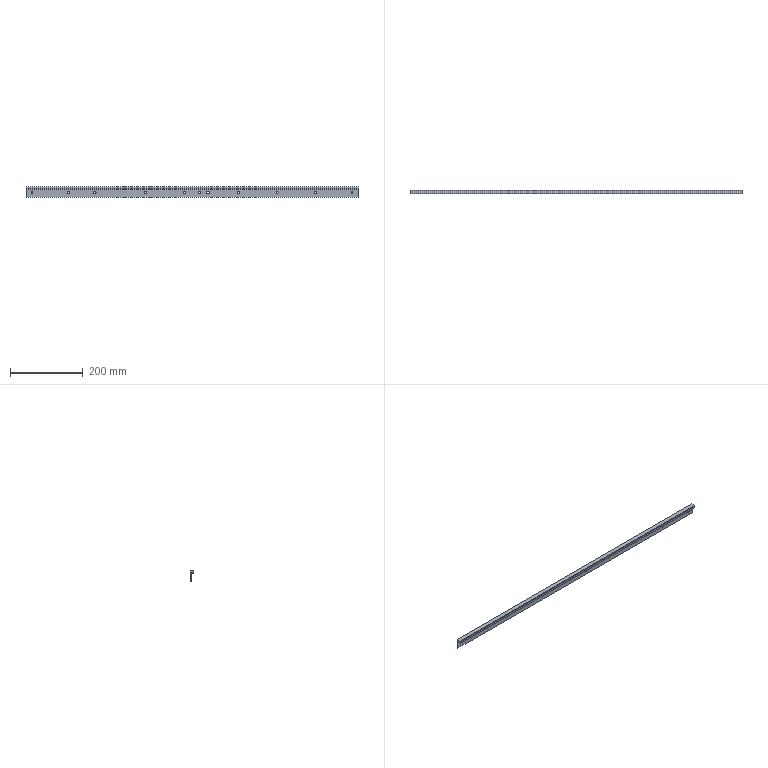Part | SolidWorks | features FlatPattern 3, SMBaseFlange 3, SheetMetal 3, HoleWzd 1, ICE 1, MoveFace 1 | 3 solids | 40 faces | box 915 x 11 x 28 mm | volume 111648 mm3 | cylinder 22 | plane 18 | commonest cylinder face diameters 5.3 x18 8 x4
STEP:
#1=CARTESIAN_POINT('',(-473.5,0.,2.65));
#2=VERTEX_POINT('',#1);
#3=CARTESIAN_POINT('',(-473.5,0.,-2.65));
#4=VERTEX_POINT('',#3);
#5=CARTESIAN_POINT('',(-473.5,0.,0.));
#6=DIRECTION('',(0.,-1.,0.));
#7=DIRECTION('',(0.,0.,-1.));
#8=AXIS2_PLACEMENT_3D('',#5,#6,#7);
#9=CIRCLE('',#8,2.65);
#10=EDGE_CURVE('',#2,#4,#9,.T.);
#11=ORIENTED_EDGE('',*,*,#10,.F.);
#12=CARTESIAN_POINT('',(-473.5,-3.,2.65));
#13=VERTEX_POINT('',#12);
#14=CARTESIAN_POINT('',(-473.5,-3.,2.65));
#15=DIRECTION('',(0.,-1.,0.));
#16=VECTOR('',#15,1000.);
#17=LINE('',#14,#16);
#18=EDGE_CURVE('',#2,#13,#17,.T.);
#19=ORIENTED_EDGE('',*,*,#18,.T.);
#20=CARTESIAN_POINT('',(-473.5,-3.,-2.65));
#21=VERTEX_POINT('',#20);
#22=CARTESIAN_POINT('',(-473.5,-3.,0.));
#23=DIRECTION('',(0.,-1.,0.));
#24=DIRECTION('',(0.,0.,-1.));
#25=AXIS2_PLACEMENT_3D('',#22,#23,#24);
#26=CIRCLE('',#25,2.65);
#27=EDGE_CURVE('',#13,#21,#26,.T.);
#28=ORIENTED_EDGE('',*,*,#27,.T.);
#29=CARTESIAN_POINT('',(-473.5,-3.,-2.65));
#30=DIRECTION('',(0.,-1.,0.));
#31=VECTOR('',#30,1000.);
#32=LINE('',#29,#31);
#33=EDGE_CURVE('',#4,#21,#32,.T.);
#34=ORIENTED_EDGE('',*,*,#33,.F.);
#35=EDGE_LOOP('',(#11,#19,#28,#34));
#36=FACE_OUTER_BOUND('',#35,.T.);
#37=CARTESIAN_POINT('',(-473.5,-3.,0.));
#38=DIRECTION('',(0.,-1.,0.));
#39=DIRECTION('',(0.,0.,-1.));
#40=AXIS2_PLACEMENT_3D('',#37,#38,#39);
#41=CYLINDRICAL_SURFACE('',#40,2.65);
#42=ADVANCED_FACE('',(#36),#41,.F.);
#43=CARTESIAN_POINT('',(-373.5,0.,2.65));
#44=VERTEX_POINT('',#43);
#45=CARTESIAN_POINT('',(-373.5,0.,-2.65));
#46=VERTEX_POINT('',#45);
#47=CARTESIAN_POINT('',(-373.5,0.,0.));
#48=DIRECTION('',(0.,-1.,0.));
#49=DIRECTION('',(0.,0.,-1.));
#50=AXIS2_PLACEMENT_3D('',#47,#48,#49);
#51=CIRCLE('',#50,2.65);
#52=EDGE_CURVE('',#44,#46,#51,.T.);
#53=ORIENTED_EDGE('',*,*,#52,.F.);
#54=CARTESIAN_POINT('',(-373.5,-3.,2.65));
#55=VERTEX_POINT('',#54);
#56=CARTESIAN_POINT('',(-373.5,-3.,2.65));
#57=DIRECTION('',(0.,-1.,0.));
#58=VECTOR('',#57,1000.);
#59=LINE('',#56,#58);
#60=EDGE_CURVE('',#44,#55,#59,.T.);
#61=ORIENTED_EDGE('',*,*,#60,.T.);
#62=CARTESIAN_POINT('',(-373.5,-3.,-2.65));
#63=VERTEX_POINT('',#62);
#64=CARTESIAN_POINT('',(-373.5,-3.,0.));
#65=DIRECTION('',(0.,-1.,0.));
#66=DIRECTION('',(0.,0.,-1.));
#67=AXIS2_PLACEMENT_3D('',#64,#65,#66);
#68=CIRCLE('',#67,2.65);
#69=EDGE_CURVE('',#55,#63,#68,.T.);
#70=ORIENTED_EDGE('',*,*,#69,.T.);
#71=CARTESIAN_POINT('',(-373.5,-3.,-2.65));
#72=DIRECTION('',(0.,-1.,0.));
#73=VECTOR('',#72,1000.);
#74=LINE('',#71,#73);
#75=EDGE_CURVE('',#46,#63,#74,.T.);
#76=ORIENTED_EDGE('',*,*,#75,.F.);
#77=EDGE_LOOP('',(#53,#61,#70,#76));
#78=FACE_OUTER_BOUND('',#77,.T.);
#79=CARTESIAN_POINT('',(-373.5,-3.,0.));
#80=DIRECTION('',(0.,-1.,0.));
#81=DIRECTION('',(0.,0.,-1.));
#82=AXIS2_PLACEMENT_3D('',#79,#80,#81);
#83=CYLINDRICAL_SURFACE('',#82,2.65);
#84=ADVANCED_FACE('',(#78),#83,.F.);
#85=CARTESIAN_POINT('',(-161.,0.,2.65));
#86=VERTEX_POINT('',#85);
#87=CARTESIAN_POINT('',(-161.,0.,-2.65));
#88=VERTEX_POINT('',#87);
#89=CARTESIAN_POINT('',(-161.,0.,0.));
#90=DIRECTION('',(0.,-1.,0.));
#91=DIRECTION('',(0.,0.,-1.));
#92=AXIS2_PLACEMENT_3D('',#89,#90,#91);
#93=CIRCLE('',#92,2.65);
#94=EDGE_CURVE('',#86,#88,#93,.T.);
#95=ORIENTED_EDGE('',*,*,#94,.F.);
#96=CARTESIAN_POINT('',(-161.,-3.,2.65));
#97=VERTEX_POINT('',#96);
#98=CARTESIAN_POINT('',(-161.,-3.,2.65));
#99=DIRECTION('',(0.,-1.,0.));
#100=VECTOR('',#99,1000.);
#101=LINE('',#98,#100);
#102=EDGE_CURVE('',#86,#97,#101,.T.);
#103=ORIENTED_EDGE('',*,*,#102,.T.);
#104=CARTESIAN_POINT('',(-161.,-3.,-2.65));
#105=VERTEX_POINT('',#104);
#106=CARTESIAN_POINT('',(-161.,-3.,0.));
#107=DIRECTION('',(0.,-1.,0.));
#108=DIRECTION('',(0.,0.,-1.));
#109=AXIS2_PLACEMENT_3D('',#106,#107,#108);
#110=CIRCLE('',#109,2.65);
#111=EDGE_CURVE('',#97,#105,#110,.T.);
#112=ORIENTED_EDGE('',*,*,#111,.T.);
#113=CARTESIAN_POINT('',(-161.,-3.,-2.65));
#114=DIRECTION('',(0.,-1.,0.));
#115=VECTOR('',#114,1000.);
#116=LINE('',#113,#115);
#117=EDGE_CURVE('',#88,#105,#116,.T.);
#118=ORIENTED_EDGE('',*,*,#117,.F.);
#119=EDGE_LOOP('',(#95,#103,#112,#118));
#120=FACE_OUTER_BOUND('',#119,.T.);
#121=CARTESIAN_POINT('',(-161.,-3.,0.));
#122=DIRECTION('',(0.,-1.,0.));
#123=DIRECTION('',(0.,0.,-1.));
#124=AXIS2_PLACEMENT_3D('',#121,#122,#123);
#125=CYLINDRICAL_SURFACE('',#124,2.65);
#126=ADVANCED_FACE('',(#120),#125,.F.);
#127=CARTESIAN_POINT('',(-53.,0.,2.65));
#128=VERTEX_POINT('',#127);
#129=CARTESIAN_POINT('',(-53.,0.,-2.65));
#130=VERTEX_POINT('',#129);
#131=CARTESIAN_POINT('',(-53.,0.,0.));
#132=DIRECTION('',(0.,-1.,0.));
#133=DIRECTION('',(0.,0.,-1.));
#134=AXIS2_PLACEMENT_3D('',#131,#132,#133);
#135=CIRCLE('',#134,2.65);
#136=EDGE_CURVE('',#128,#130,#135,.T.);
#137=ORIENTED_EDGE('',*,*,#136,.F.);
#138=CARTESIAN_POINT('',(-53.,-3.,2.65));
#139=VERTEX_POINT('',#138);
#140=CARTESIAN_POINT('',(-53.,-3.,2.65));
#141=DIRECTION('',(0.,-1.,0.));
#142=VECTOR('',#141,1000.);
#143=LINE('',#140,#142);
#144=EDGE_CURVE('',#128,#139,#143,.T.);
#145=ORIENTED_EDGE('',*,*,#144,.T.);
#146=CARTESIAN_POINT('',(-53.,-3.,-2.65));
#147=VERTEX_POINT('',#146);
#148=CARTESIAN_POINT('',(-53.,-3.,0.));
#149=DIRECTION('',(0.,-1.,0.));
#150=DIRECTION('',(0.,0.,-1.));
#151=AXIS2_PLACEMENT_3D('',#148,#149,#150);
#152=CIRCLE('',#151,2.65);
#153=EDGE_CURVE('',#139,#147,#152,.T.);
#154=ORIENTED_EDGE('',*,*,#153,.T.);
#155=CARTESIAN_POINT('',(-53.,-3.,-2.65));
#156=DIRECTION('',(0.,-1.,0.));
#157=VECTOR('',#156,1000.);
#158=LINE('',#155,#157);
#159=EDGE_CURVE('',#130,#147,#158,.T.);
#160=ORIENTED_EDGE('',*,*,#159,.F.);
#161=EDGE_LOOP('',(#137,#145,#154,#160));
#162=FACE_OUTER_BOUND('',#161,.T.);
#163=CARTESIAN_POINT('',(-53.,-3.,0.));
#164=DIRECTION('',(0.,-1.,0.));
#165=DIRECTION('',(0.,0.,-1.));
#166=AXIS2_PLACEMENT_3D('',#163,#164,#165);
#167=CYLINDRICAL_SURFACE('',#166,2.65);
#168=ADVANCED_FACE('',(#162),#167,.F.);
#169=CARTESIAN_POINT('',(-12.,0.,2.65));
#170=VERTEX_POINT('',#169);
#171=CARTESIAN_POINT('',(-12.,0.,-2.65));
#172=VERTEX_POINT('',#171);
#173=CARTESIAN_POINT('',(-12.,0.,0.));
#174=DIRECTION('',(0.,-1.,0.));
#175=DIRECTION('',(0.,0.,-1.));
#176=AXIS2_PLACEMENT_3D('',#173,#174,#175);
#177=CIRCLE('',#176,2.65);
#178=EDGE_CURVE('',#170,#172,#177,.T.);
#179=ORIENTED_EDGE('',*,*,#178,.F.);
#180=CARTESIAN_POINT('',(-12.,-3.,2.65));
#181=VERTEX_POINT('',#180);
#182=CARTESIAN_POINT('',(-12.,-3.,2.65));
#183=DIRECTION('',(0.,-1.,0.));
#184=VECTOR('',#183,1000.);
#185=LINE('',#182,#184);
#186=EDGE_CURVE('',#170,#181,#185,.T.);
#187=ORIENTED_EDGE('',*,*,#186,.T.);
#188=CARTESIAN_POINT('',(-12.,-3.,-2.65));
#189=VERTEX_POINT('',#188);
#190=CARTESIAN_POINT('',(-12.,-3.,0.));
#191=DIRECTION('',(0.,-1.,0.));
#192=DIRECTION('',(0.,0.,-1.));
#193=AXIS2_PLACEMENT_3D('',#190,#191,#192);
#194=CIRCLE('',#193,2.65);
#195=EDGE_CURVE('',#181,#189,#194,.T.);
#196=ORIENTED_EDGE('',*,*,#195,.T.);
#197=CARTESIAN_POINT('',(-12.,-3.,-2.65));
#198=DIRECTION('',(0.,-1.,0.));
#199=VECTOR('',#198,1000.);
#200=LINE('',#197,#199);
#201=EDGE_CURVE('',#172,#189,#200,.T.);
#202=ORIENTED_EDGE('',*,*,#201,.F.);
#203=EDGE_LOOP('',(#179,#187,#196,#202));
#204=FACE_OUTER_BOUND('',#203,.T.);
#205=CARTESIAN_POINT('',(-12.,-3.,0.));
#206=DIRECTION('',(0.,-1.,0.));
#207=DIRECTION('',(0.,0.,-1.));
#208=AXIS2_PLACEMENT_3D('',#205,#206,#207);
#209=CYLINDRICAL_SURFACE('',#208,2.65);
#210=ADVANCED_FACE('',(#204),#209,.F.);
#211=CARTESIAN_POINT('',(96.,0.,2.65));
#212=VERTEX_POINT('',#211);
#213=CARTESIAN_POINT('',(96.,0.,-2.65));
#214=VERTEX_POINT('',#213);
#215=CARTESIAN_POINT('',(96.,0.,0.));
#216=DIRECTION('',(0.,-1.,0.));
#217=DIRECTION('',(0.,0.,-1.));
#218=AXIS2_PLACEMENT_3D('',#215,#216,#217);
#219=CIRCLE('',#218,2.65);
#220=EDGE_CURVE('',#212,#214,#219,.T.);
#221=ORIENTED_EDGE('',*,*,#220,.F.);
#222=CARTESIAN_POINT('',(96.,-3.,2.65));
#223=VERTEX_POINT('',#222);
#224=CARTESIAN_POINT('',(96.,-3.,2.65));
#225=DIRECTION('',(0.,-1.,0.));
#226=VECTOR('',#225,1000.);
#227=LINE('',#224,#226);
#228=EDGE_CURVE('',#212,#223,#227,.T.);
#229=ORIENTED_EDGE('',*,*,#228,.T.);
#230=CARTESIAN_POINT('',(96.,-3.,-2.65));
#231=VERTEX_POINT('',#230);
#232=CARTESIAN_POINT('',(96.,-3.,0.));
#233=DIRECTION('',(0.,-1.,0.));
#234=DIRECTION('',(0.,0.,-1.));
#235=AXIS2_PLACEMENT_3D('',#232,#233,#234);
#236=CIRCLE('',#235,2.65);
#237=EDGE_CURVE('',#223,#231,#236,.T.);
#238=ORIENTED_EDGE('',*,*,#237,.T.);
#239=CARTESIAN_POINT('',(96.,-3.,-2.65));
#240=DIRECTION('',(0.,-1.,0.));
#241=VECTOR('',#240,1000.);
#242=LINE('',#239,#241);
#243=EDGE_CURVE('',#214,#231,#242,.T.);
#244=ORIENTED_EDGE('',*,*,#243,.F.);
#245=EDGE_LOOP('',(#221,#229,#238,#244));
#246=FACE_OUTER_BOUND('',#245,.T.);
#247=CARTESIAN_POINT('',(96.,-3.,0.));
#248=DIRECTION('',(0.,-1.,0.));
#249=DIRECTION('',(0.,0.,-1.));
#250=AXIS2_PLACEMENT_3D('',#247,#248,#249);
#251=CYLINDRICAL_SURFACE('',#250,2.65);
#252=ADVANCED_FACE('',(#246),#251,.F.);
#253=CARTESIAN_POINT('',(202.25,0.,2.65));
#254=VERTEX_POINT('',#253);
#255=CARTESIAN_POINT('',(202.25,0.,-2.65));
#256=VERTEX_POINT('',#255);
#257=CARTESIAN_POINT('',(202.25,0.,0.));
#258=DIRECTION('',(0.,-1.,0.));
#259=DIRECTION('',(0.,0.,-1.));
#260=AXIS2_PLACEMENT_3D('',#257,#258,#259);
#261=CIRCLE('',#260,2.65);
#262=EDGE_CURVE('',#254,#256,#261,.T.);
#263=ORIENTED_EDGE('',*,*,#262,.F.);
#264=CARTESIAN_POINT('',(202.25,-3.,2.65));
#265=VERTEX_POINT('',#264);
#266=CARTESIAN_POINT('',(202.25,-3.,2.65));
#267=DIRECTION('',(0.,-1.,0.));
#268=VECTOR('',#267,1000.);
#269=LINE('',#266,#268);
#270=EDGE_CURVE('',#254,#265,#269,.T.);
#271=ORIENTED_EDGE('',*,*,#270,.T.);
#272=CARTESIAN_POINT('',(202.25,-3.,-2.65));
#273=VERTEX_POINT('',#272);
#274=CARTESIAN_POINT('',(202.25,-3.,0.));
#275=DIRECTION('',(0.,-1.,0.));
#276=DIRECTION('',(0.,0.,-1.));
#277=AXIS2_PLACEMENT_3D('',#274,#275,#276);
#278=CIRCLE('',#277,2.65);
#279=EDGE_CURVE('',#265,#273,#278,.T.);
#280=ORIENTED_EDGE('',*,*,#279,.T.);
#281=CARTESIAN_POINT('',(202.25,-3.,-2.65));
#282=DIRECTION('',(0.,-1.,0.));
#283=VECTOR('',#282,1000.);
#284=LINE('',#281,#283);
#285=EDGE_CURVE('',#256,#273,#284,.T.);
#286=ORIENTED_EDGE('',*,*,#285,.F.);
#287=EDGE_LOOP('',(#263,#271,#280,#286));
#288=FACE_OUTER_BOUND('',#287,.T.);
#289=CARTESIAN_POINT('',(202.25,-3.,0.));
#290=DIRECTION('',(0.,-1.,0.));
#291=DIRECTION('',(0.,0.,-1.));
#292=AXIS2_PLACEMENT_3D('',#289,#290,#291);
#293=CYLINDRICAL_SURFACE('',#292,2.65);
#294=ADVANCED_FACE('',(#288),#293,.F.);
#295=CARTESIAN_POINT('',(308.5,0.,2.65));
#296=VERTEX_POINT('',#295);
#297=CARTESIAN_POINT('',(308.5,0.,-2.65));
#298=VERTEX_POINT('',#297);
#299=CARTESIAN_POINT('',(308.5,0.,0.));
#300=DIRECTION('',(0.,-1.,0.));
#301=DIRECTION('',(0.,0.,-1.));
#302=AXIS2_PLACEMENT_3D('',#299,#300,#301);
#303=CIRCLE('',#302,2.65);
#304=EDGE_CURVE('',#296,#298,#303,.T.);
#305=ORIENTED_EDGE('',*,*,#304,.F.);
#306=CARTESIAN_POINT('',(308.5,-3.,2.65));
#307=VERTEX_POINT('',#306);
#308=CARTESIAN_POINT('',(308.5,-3.,2.65));
#309=DIRECTION('',(0.,-1.,0.));
#310=VECTOR('',#309,1000.);
#311=LINE('',#308,#310);
#312=EDGE_CURVE('',#296,#307,#311,.T.);
#313=ORIENTED_EDGE('',*,*,#312,.T.);
#314=CARTESIAN_POINT('',(308.5,-3.,-2.65));
#315=VERTEX_POINT('',#314);
#316=CARTESIAN_POINT('',(308.5,-3.,0.));
#317=DIRECTION('',(0.,-1.,0.));
#318=DIRECTION('',(0.,0.,-1.));
#319=AXIS2_PLACEMENT_3D('',#316,#317,#318);
#320=CIRCLE('',#319,2.65);
#321=EDGE_CURVE('',#307,#315,#320,.T.);
#322=ORIENTED_EDGE('',*,*,#321,.T.);
#323=CARTESIAN_POINT('',(308.5,-3.,-2.65));
#324=DIRECTION('',(0.,-1.,0.));
#325=VECTOR('',#324,1000.);
#326=LINE('',#323,#325);
#327=EDGE_CURVE('',#298,#315,#326,.T.);
#328=ORIENTED_EDGE('',*,*,#327,.F.);
#329=EDGE_LOOP('',(#305,#313,#322,#328));
#330=FACE_OUTER_BOUND('',#329,.T.);
#331=CARTESIAN_POINT('',(308.5,-3.,0.));
#332=DIRECTION('',(0.,-1.,0.));
#333=DIRECTION('',(0.,0.,-1.));
#334=AXIS2_PLACEMENT_3D('',#331,#332,#333);
#335=CYLINDRICAL_SURFACE('',#334,2.65);
#336=ADVANCED_FACE('',(#330),#335,.F.);
#337=CARTESIAN_POINT('',(408.5,0.,2.65));
#338=VERTEX_POINT('',#337);
#339=CARTESIAN_POINT('',(408.5,0.,-2.65));
#340=VERTEX_POINT('',#339);
#341=CARTESIAN_POINT('',(408.5,0.,0.));
#342=DIRECTION('',(0.,-1.,0.));
#343=DIRECTION('',(0.,0.,-1.));
#344=AXIS2_PLACEMENT_3D('',#341,#342,#343);
#345=CIRCLE('',#344,2.65);
#346=EDGE_CURVE('',#338,#340,#345,.T.);
#347=ORIENTED_EDGE('',*,*,#346,.F.);
#348=CARTESIAN_POINT('',(408.5,-3.,2.65));
#349=VERTEX_POINT('',#348);
#350=CARTESIAN_POINT('',(408.5,-3.,2.65));
#351=DIRECTION('',(0.,-1.,0.));
#352=VECTOR('',#351,1000.);
#353=LINE('',#350,#352);
#354=EDGE_CURVE('',#338,#349,#353,.T.);
#355=ORIENTED_EDGE('',*,*,#354,.T.);
#356=CARTESIAN_POINT('',(408.5,-3.,-2.65));
#357=VERTEX_POINT('',#356);
#358=CARTESIAN_POINT('',(408.5,-3.,0.));
#359=DIRECTION('',(0.,-1.,0.));
#360=DIRECTION('',(0.,0.,-1.));
#361=AXIS2_PLACEMENT_3D('',#358,#359,#360);
#362=CIRCLE('',#361,2.65);
#363=EDGE_CURVE('',#349,#357,#362,.T.);
#364=ORIENTED_EDGE('',*,*,#363,.T.);
#365=CARTESIAN_POINT('',(408.5,-3.,-2.65));
#366=DIRECTION('',(0.,-1.,0.));
#367=VECTOR('',#366,1000.);
#368=LINE('',#365,#367);
#369=EDGE_CURVE('',#340,#357,#368,.T.);
#370=ORIENTED_EDGE('',*,*,#369,.F.);
#371=EDGE_LOOP('',(#347,#355,#364,#370));
#372=FACE_OUTER_BOUND('',#371,.T.);
#373=CARTESIAN_POINT('',(408.5,-3.,0.));
#374=DIRECTION('',(0.,-1.,0.));
#375=DIRECTION('',(0.,0.,-1.));
#376=AXIS2_PLACEMENT_3D('',#373,#374,#375);
#377=CYLINDRICAL_SURFACE('',#376,2.65);
#378=ADVANCED_FACE('',(#372),#377,.F.);
#379=CARTESIAN_POINT('',(11.5,0.,4.));
#380=VERTEX_POINT('',#379);
#381=CARTESIAN_POINT('',(11.5,0.,-4.));
#382=VERTEX_POINT('',#381);
#383=CARTESIAN_POINT('',(11.5,0.,0.));
#384=DIRECTION('',(0.,-1.,0.));
#385=DIRECTION('',(0.,0.,-1.));
#386=AXIS2_PLACEMENT_3D('',#383,#384,#385);
#387=CIRCLE('',#386,4.);
#388=EDGE_CURVE('',#380,#382,#387,.T.);
#389=ORIENTED_EDGE('',*,*,#388,.F.);
#390=CARTESIAN_POINT('',(11.5,-3.,4.));
#391=VERTEX_POINT('',#390);
#392=CARTESIAN_POINT('',(11.5,0.,4.));
#393=DIRECTION('',(0.,-1.,0.));
#394=VECTOR('',#393,1000.);
#395=LINE('',#392,#394);
#396=EDGE_CURVE('',#380,#391,#395,.T.);
#397=ORIENTED_EDGE('',*,*,#396,.T.);
#398=CARTESIAN_POINT('',(11.5,-3.,-4.));
#399=VERTEX_POINT('',#398);
#400=CARTESIAN_POINT('',(11.5,-3.,0.));
#401=DIRECTION('',(0.,-1.,0.));
#402=DIRECTION('',(0.,0.,-1.));
#403=AXIS2_PLACEMENT_3D('',#400,#401,#402);
#404=CIRCLE('',#403,4.);
#405=EDGE_CURVE('',#391,#399,#404,.T.);
#406=ORIENTED_EDGE('',*,*,#405,.T.);
#407=CARTESIAN_POINT('',(11.5,0.,-4.));
#408=DIRECTION('',(0.,-1.,0.));
#409=VECTOR('',#408,1000.);
#410=LINE('',#407,#409);
#411=EDGE_CURVE('',#382,#399,#410,.T.);
#412=ORIENTED_EDGE('',*,*,#411,.F.);
#413=EDGE_LOOP('',(#389,#397,#406,#412));
#414=FACE_OUTER_BOUND('',#413,.T.);
#415=CARTESIAN_POINT('',(11.5,0.,0.));
#416=DIRECTION('',(0.,-1.,0.));
#417=DIRECTION('',(0.,0.,-1.));
#418=AXIS2_PLACEMENT_3D('',#415,#416,#417);
#419=CYLINDRICAL_SURFACE('',#418,4.);
#420=ADVANCED_FACE('',(#414),#419,.F.);
#421=CARTESIAN_POINT('',(-301.,0.,4.));
#422=VERTEX_POINT('',#421);
#423=CARTESIAN_POINT('',(-301.,0.,-4.));
#424=VERTEX_POINT('',#423);
#425=CARTESIAN_POINT('',(-301.,0.,0.));
#426=DIRECTION('',(0.,-1.,0.));
#427=DIRECTION('',(0.,0.,-1.));
#428=AXIS2_PLACEMENT_3D('',#425,#426,#427);
#429=CIRCLE('',#428,4.);
#430=EDGE_CURVE('',#422,#424,#429,.T.);
#431=ORIENTED_EDGE('',*,*,#430,.F.);
#432=CARTESIAN_POINT('',(-301.,-3.,4.));
#433=VERTEX_POINT('',#432);
#434=CARTESIAN_POINT('',(-301.,0.,4.));
#435=DIRECTION('',(0.,-1.,0.));
#436=VECTOR('',#435,1000.);
#437=LINE('',#434,#436);
#438=EDGE_CURVE('',#422,#433,#437,.T.);
#439=ORIENTED_EDGE('',*,*,#438,.T.);
#440=CARTESIAN_POINT('',(-301.,-3.,-4.));
#441=VERTEX_POINT('',#440);
#442=CARTESIAN_POINT('',(-301.,-3.,0.));
#443=DIRECTION('',(0.,-1.,0.));
#444=DIRECTION('',(0.,0.,-1.));
#445=AXIS2_PLACEMENT_3D('',#442,#443,#444);
#446=CIRCLE('',#445,4.);
#447=EDGE_CURVE('',#433,#441,#446,.T.);
#448=ORIENTED_EDGE('',*,*,#447,.T.);
#449=CARTESIAN_POINT('',(-301.,0.,-4.));
#450=DIRECTION('',(0.,-1.,0.));
#451=VECTOR('',#450,1000.);
#452=LINE('',#449,#451);
#453=EDGE_CURVE('',#424,#441,#452,.T.);
#454=ORIENTED_EDGE('',*,*,#453,.F.);
#455=EDGE_LOOP('',(#431,#439,#448,#454));
#456=FACE_OUTER_BOUND('',#455,.T.);
#457=CARTESIAN_POINT('',(-301.,0.,0.));
#458=DIRECTION('',(0.,-1.,0.));
#459=DIRECTION('',(0.,0.,-1.));
#460=AXIS2_PLACEMENT_3D('',#457,#458,#459);
#461=CYLINDRICAL_SURFACE('',#460,4.);
#462=ADVANCED_FACE('',(#456),#461,.F.);
#463=CARTESIAN_POINT('',(-473.5,0.,0.));
#464=DIRECTION('',(0.,-1.,0.));
#465=DIRECTION('',(0.,0.,-1.));
#466=AXIS2_PLACEMENT_3D('',#463,#464,#465);
#467=CIRCLE('',#466,2.65);
#468=EDGE_CURVE('',#4,#2,#467,.T.);
#469=ORIENTED_EDGE('',*,*,#468,.T.);
#470=ORIENTED_EDGE('',*,*,#10,.T.);
#471=EDGE_LOOP('',(#469,#470));
#472=FACE_BOUND('',#471,.T.);
#473=CARTESIAN_POINT('',(-373.5,0.,0.));
#474=DIRECTION('',(0.,-1.,0.));
#475=DIRECTION('',(0.,0.,-1.));
#476=AXIS2_PLACEMENT_3D('',#473,#474,#475);
#477=CIRCLE('',#476,2.65);
#478=EDGE_CURVE('',#46,#44,#477,.T.);
#479=ORIENTED_EDGE('',*,*,#478,.T.);
#480=ORIENTED_EDGE('',*,*,#52,.T.);
#481=EDGE_LOOP('',(#479,#480));
#482=FACE_BOUND('',#481,.T.);
#483=CARTESIAN_POINT('',(-161.,0.,0.));
#484=DIRECTION('',(0.,-1.,0.));
#485=DIRECTION('',(0.,0.,-1.));
#486=AXIS2_PLACEMENT_3D('',#483,#484,#485);
#487=CIRCLE('',#486,2.65);
#488=EDGE_CURVE('',#88,#86,#487,.T.);
#489=ORIENTED_EDGE('',*,*,#488,.T.);
#490=ORIENTED_EDGE('',*,*,#94,.T.);
#491=EDGE_LOOP('',(#489,#490));
#492=FACE_BOUND('',#491,.T.);
#493=CARTESIAN_POINT('',(-53.,0.,0.));
#494=DIRECTION('',(0.,-1.,0.));
#495=DIRECTION('',(0.,0.,-1.));
#496=AXIS2_PLACEMENT_3D('',#493,#494,#495);
#497=CIRCLE('',#496,2.65);
#498=EDGE_CURVE('',#130,#128,#497,.T.);
#499=ORIENTED_EDGE('',*,*,#498,.T.);
#500=ORIENTED_EDGE('',*,*,#136,.T.);
#501=EDGE_LOOP('',(#499,#500));
#502=FACE_BOUND('',#501,.T.);
#503=CARTESIAN_POINT('',(425.,0.,12.5));
#504=VERTEX_POINT('',#503);
#505=CARTESIAN_POINT('',(425.,0.,-12.5));
#506=VERTEX_POINT('',#505);
#507=CARTESIAN_POINT('',(425.,0.,-12.5));
#508=DIRECTION('',(0.,0.,-1.));
#509=VECTOR('',#508,1000.);
#510=LINE('',#507,#509);
#511=EDGE_CURVE('',#504,#506,#510,.T.);
#512=ORIENTED_EDGE('',*,*,#511,.T.);
#513=CARTESIAN_POINT('',(-490.,0.,-12.5));
#514=VERTEX_POINT('',#513);
#515=CARTESIAN_POINT('',(-425.,0.,-12.5));
#516=DIRECTION('',(-1.,0.,0.));
#517=VECTOR('',#516,1000.);
#518=LINE('',#515,#517);
#519=EDGE_CURVE('',#506,#514,#518,.T.);
#520=ORIENTED_EDGE('',*,*,#519,.T.);
#521=CARTESIAN_POINT('',(-490.,0.,12.5));
#522=VERTEX_POINT('',#521);
#523=CARTESIAN_POINT('',(-490.,0.,-12.5));
#524=DIRECTION('',(0.,0.,1.));
#525=VECTOR('',#524,1000.);
#526=LINE('',#523,#525);
#527=EDGE_CURVE('',#514,#522,#526,.T.);
#528=ORIENTED_EDGE('',*,*,#527,.T.);
#529=CARTESIAN_POINT('',(-425.,0.,12.5));
#530=DIRECTION('',(1.,0.,0.));
#531=VECTOR('',#530,1000.);
#532=LINE('',#529,#531);
#533=EDGE_CURVE('',#522,#504,#532,.T.);
#534=ORIENTED_EDGE('',*,*,#533,.T.);
#535=EDGE_LOOP('',(#512,#520,#528,#534));
#536=FACE_OUTER_BOUND('',#535,.T.);
#537=CARTESIAN_POINT('',(-301.,0.,0.));
#538=DIRECTION('',(0.,-1.,0.));
#539=DIRECTION('',(0.,0.,-1.));
#540=AXIS2_PLACEMENT_3D('',#537,#538,#539);
#541=CIRCLE('',#540,4.);
#542=EDGE_CURVE('',#424,#422,#541,.T.);
#543=ORIENTED_EDGE('',*,*,#542,.T.);
#544=ORIENTED_EDGE('',*,*,#430,.T.);
#545=EDGE_LOOP('',(#543,#544));
#546=FACE_BOUND('',#545,.T.);
#547=CARTESIAN_POINT('',(11.5,0.,0.));
#548=DIRECTION('',(0.,-1.,0.));
#549=DIRECTION('',(0.,0.,-1.));
#550=AXIS2_PLACEMENT_3D('',#547,#548,#549);
#551=CIRCLE('',#550,4.);
#552=EDGE_CURVE('',#382,#380,#551,.T.);
#553=ORIENTED_EDGE('',*,*,#552,.T.);
#554=ORIENTED_EDGE('',*,*,#388,.T.);
#555=EDGE_LOOP('',(#553,#554));
#556=FACE_BOUND('',#555,.T.);
#557=CARTESIAN_POINT('',(408.5,0.,0.));
#558=DIRECTION('',(0.,-1.,0.));
#559=DIRECTION('',(0.,0.,-1.));
#560=AXIS2_PLACEMENT_3D('',#557,#558,#559);
#561=CIRCLE('',#560,2.65);
#562=EDGE_CURVE('',#340,#338,#561,.T.);
#563=ORIENTED_EDGE('',*,*,#562,.T.);
#564=ORIENTED_EDGE('',*,*,#346,.T.);
#565=EDGE_LOOP('',(#563,#564));
#566=FACE_BOUND('',#565,.T.);
#567=CARTESIAN_POINT('',(308.5,0.,0.));
#568=DIRECTION('',(0.,-1.,0.));
#569=DIRECTION('',(0.,0.,-1.));
#570=AXIS2_PLACEMENT_3D('',#567,#568,#569);
#571=CIRCLE('',#570,2.65);
#572=EDGE_CURVE('',#298,#296,#571,.T.);
#573=ORIENTED_EDGE('',*,*,#572,.T.);
#574=ORIENTED_EDGE('',*,*,#304,.T.);
#575=EDGE_LOOP('',(#573,#574));
#576=FACE_BOUND('',#575,.T.);
#577=CARTESIAN_POINT('',(202.25,0.,0.));
#578=DIRECTION('',(0.,-1.,0.));
#579=DIRECTION('',(0.,0.,-1.));
#580=AXIS2_PLACEMENT_3D('',#577,#578,#579);
#581=CIRCLE('',#580,2.65);
#582=EDGE_CURVE('',#256,#254,#581,.T.);
#583=ORIENTED_EDGE('',*,*,#582,.T.);
#584=ORIENTED_EDGE('',*,*,#262,.T.);
#585=EDGE_LOOP('',(#583,#584));
#586=FACE_BOUND('',#585,.T.);
#587=CARTESIAN_POINT('',(96.,0.,0.));
#588=DIRECTION('',(0.,-1.,0.));
#589=DIRECTION('',(0.,0.,-1.));
#590=AXIS2_PLACEMENT_3D('',#587,#588,#589);
#591=CIRCLE('',#590,2.65);
#592=EDGE_CURVE('',#214,#212,#591,.T.);
#593=ORIENTED_EDGE('',*,*,#592,.T.);
#594=ORIENTED_EDGE('',*,*,#220,.T.);
#595=EDGE_LOOP('',(#593,#594));
#596=FACE_BOUND('',#595,.T.);
#597=CARTESIAN_POINT('',(-12.,0.,0.));
#598=DIRECTION('',(0.,-1.,0.));
#599=DIRECTION('',(0.,0.,-1.));
#600=AXIS2_PLACEMENT_3D('',#597,#598,#599);
#601=CIRCLE('',#600,2.65);
#602=EDGE_CURVE('',#172,#170,#601,.T.);
#603=ORIENTED_EDGE('',*,*,#602,.T.);
#604=ORIENTED_EDGE('',*,*,#178,.T.);
#605=EDGE_LOOP('',(#603,#604));
#606=FACE_BOUND('',#605,.T.);
#607=CARTESIAN_POINT('',(0.,0.,0.));
#608=DIRECTION('',(0.,1.,0.));
#609=DIRECTION('',(0.,0.,1.));
#610=AXIS2_PLACEMENT_3D('',#607,#608,#609);
#611=PLANE('',#610);
#612=ADVANCED_FACE('',(#472,#482,#492,#502,#536,#546,#556,#566,#576,#586,#596,#606),#611,.T.);
#613=ORIENTED_EDGE('',*,*,#511,.F.);
#614=CARTESIAN_POINT('',(425.,-3.,12.5));
#615=VERTEX_POINT('',#614);
#616=CARTESIAN_POINT('',(425.,-3.,12.5));
#617=DIRECTION('',(0.,1.,0.));
#618=VECTOR('',#617,1000.);
#619=LINE('',#616,#618);
#620=EDGE_CURVE('',#615,#504,#619,.T.);
#621=ORIENTED_EDGE('',*,*,#620,.F.);
#622=CARTESIAN_POINT('',(425.,-3.,-12.5));
#623=VERTEX_POINT('',#622);
#624=CARTESIAN_POINT('',(425.,-3.,-12.5));
#625=DIRECTION('',(0.,0.,-1.));
#626=VECTOR('',#625,1000.);
#627=LINE('',#624,#626);
#628=EDGE_CURVE('',#615,#623,#627,.T.);
#629=ORIENTED_EDGE('',*,*,#628,.T.);
#630=CARTESIAN_POINT('',(425.,-3.,-12.5));
#631=DIRECTION('',(0.,1.,0.));
#632=VECTOR('',#631,1000.);
#633=LINE('',#630,#632);
#634=EDGE_CURVE('',#623,#506,#633,.T.);
#635=ORIENTED_EDGE('',*,*,#634,.T.);
#636=EDGE_LOOP('',(#613,#621,#629,#635));
#637=FACE_OUTER_BOUND('',#636,.T.);
#638=CARTESIAN_POINT('',(425.,-3.,-12.5));
#639=DIRECTION('',(1.,0.,0.));
#640=DIRECTION('',(0.,0.,-1.));
#641=AXIS2_PLACEMENT_3D('',#638,#639,#640);
#642=PLANE('',#641);
#643=ADVANCED_FACE('',(#637),#642,.T.);
#644=ORIENTED_EDGE('',*,*,#533,.F.);
#645=CARTESIAN_POINT('',(-490.,-3.,12.5));
#646=VERTEX_POINT('',#645);
#647=CARTESIAN_POINT('',(-490.,-3.,12.5));
#648=DIRECTION('',(0.,1.,0.));
#649=VECTOR('',#648,1000.);
#650=LINE('',#647,#649);
#651=EDGE_CURVE('',#646,#522,#650,.T.);
#652=ORIENTED_EDGE('',*,*,#651,.F.);
#653=CARTESIAN_POINT('',(-425.,-3.,12.5));
#654=DIRECTION('',(1.,0.,0.));
#655=VECTOR('',#654,1000.);
#656=LINE('',#653,#655);
#657=EDGE_CURVE('',#646,#615,#656,.T.);
#658=ORIENTED_EDGE('',*,*,#657,.T.);
#659=ORIENTED_EDGE('',*,*,#620,.T.);
#660=EDGE_LOOP('',(#644,#652,#658,#659));
#661=FACE_OUTER_BOUND('',#660,.T.);
#662=CARTESIAN_POINT('',(-425.,-3.,12.5));
#663=DIRECTION('',(0.,0.,1.));
#664=DIRECTION('',(1.,0.,0.));
#665=AXIS2_PLACEMENT_3D('',#662,#663,#664);
#666=PLANE('',#665);
#667=ADVANCED_FACE('',(#661),#666,.T.);
#668=ORIENTED_EDGE('',*,*,#527,.F.);
#669=CARTESIAN_POINT('',(-490.,-3.,-12.5));
#670=VERTEX_POINT('',#669);
#671=CARTESIAN_POINT('',(-490.,-3.,-12.5));
#672=DIRECTION('',(0.,1.,0.));
#673=VECTOR('',#672,1000.);
#674=LINE('',#671,#673);
#675=EDGE_CURVE('',#670,#514,#674,.T.);
#676=ORIENTED_EDGE('',*,*,#675,.F.);
#677=CARTESIAN_POINT('',(-490.,-3.,-12.5));
#678=DIRECTION('',(0.,0.,1.));
#679=VECTOR('',#678,1000.);
#680=LINE('',#677,#679);
#681=EDGE_CURVE('',#670,#646,#680,.T.);
#682=ORIENTED_EDGE('',*,*,#681,.T.);
#683=ORIENTED_EDGE('',*,*,#651,.T.);
#684=EDGE_LOOP('',(#668,#676,#682,#683));
#685=FACE_OUTER_BOUND('',#684,.T.);
#686=CARTESIAN_POINT('',(-490.,-3.,-12.5));
#687=DIRECTION('',(-1.,0.,0.));
#688=DIRECTION('',(0.,0.,1.));
#689=AXIS2_PLACEMENT_3D('',#686,#687,#688);
#690=PLANE('',#689);
#691=ADVANCED_FACE('',(#685),#690,.T.);
#692=ORIENTED_EDGE('',*,*,#519,.F.);
#693=ORIENTED_EDGE('',*,*,#634,.F.);
#694=CARTESIAN_POINT('',(-425.,-3.,-12.5));
#695=DIRECTION('',(-1.,0.,0.));
#696=VECTOR('',#695,1000.);
#697=LINE('',#694,#696);
#698=EDGE_CURVE('',#623,#670,#697,.T.);
#699=ORIENTED_EDGE('',*,*,#698,.T.);
#700=ORIENTED_EDGE('',*,*,#675,.T.);
#701=EDGE_LOOP('',(#692,#693,#699,#700));
#702=FACE_OUTER_BOUND('',#701,.T.);
#703=CARTESIAN_POINT('',(-425.,-3.,-12.5));
#704=DIRECTION('',(0.,0.,-1.));
#705=DIRECTION('',(-1.,0.,0.));
#706=AXIS2_PLACEMENT_3D('',#703,#704,#705);
#707=PLANE('',#706);
#708=ADVANCED_FACE('',(#702),#707,.T.);
#709=CARTESIAN_POINT('',(-473.5,-3.,0.));
#710=DIRECTION('',(0.,-1.,0.));
#711=DIRECTION('',(0.,0.,-1.));
#712=AXIS2_PLACEMENT_3D('',#709,#710,#711);
#713=CIRCLE('',#712,2.65);
#714=EDGE_CURVE('',#21,#13,#713,.T.);
#715=ORIENTED_EDGE('',*,*,#714,.F.);
#716=ORIENTED_EDGE('',*,*,#27,.F.);
#717=EDGE_LOOP('',(#715,#716));
#718=FACE_BOUND('',#717,.T.);
#719=CARTESIAN_POINT('',(-373.5,-3.,0.));
#720=DIRECTION('',(0.,-1.,0.));
#721=DIRECTION('',(0.,0.,-1.));
#722=AXIS2_PLACEMENT_3D('',#719,#720,#721);
#723=CIRCLE('',#722,2.65);
#724=EDGE_CURVE('',#63,#55,#723,.T.);
#725=ORIENTED_EDGE('',*,*,#724,.F.);
#726=ORIENTED_EDGE('',*,*,#69,.F.);
#727=EDGE_LOOP('',(#725,#726));
#728=FACE_BOUND('',#727,.T.);
#729=CARTESIAN_POINT('',(-161.,-3.,0.));
#730=DIRECTION('',(0.,-1.,0.));
#731=DIRECTION('',(0.,0.,-1.));
#732=AXIS2_PLACEMENT_3D('',#729,#730,#731);
#733=CIRCLE('',#732,2.65);
#734=EDGE_CURVE('',#105,#97,#733,.T.);
#735=ORIENTED_EDGE('',*,*,#734,.F.);
#736=ORIENTED_EDGE('',*,*,#111,.F.);
#737=EDGE_LOOP('',(#735,#736));
#738=FACE_BOUND('',#737,.T.);
#739=CARTESIAN_POINT('',(-53.,-3.,0.));
#740=DIRECTION('',(0.,-1.,0.));
#741=DIRECTION('',(0.,0.,-1.));
#742=AXIS2_PLACEMENT_3D('',#739,#740,#741);
#743=CIRCLE('',#742,2.65);
#744=EDGE_CURVE('',#147,#139,#743,.T.);
#745=ORIENTED_EDGE('',*,*,#744,.F.);
#746=ORIENTED_EDGE('',*,*,#153,.F.);
#747=EDGE_LOOP('',(#745,#746));
#748=FACE_BOUND('',#747,.T.);
#749=CARTESIAN_POINT('',(-12.,-3.,0.));
#750=DIRECTION('',(0.,-1.,0.));
#751=DIRECTION('',(0.,0.,-1.));
#752=AXIS2_PLACEMENT_3D('',#749,#750,#751);
#753=CIRCLE('',#752,2.65);
#754=EDGE_CURVE('',#189,#181,#753,.T.);
#755=ORIENTED_EDGE('',*,*,#754,.F.);
#756=ORIENTED_EDGE('',*,*,#195,.F.);
#757=EDGE_LOOP('',(#755,#756));
#758=FACE_BOUND('',#757,.T.);
#759=CARTESIAN_POINT('',(96.,-3.,0.));
#760=DIRECTION('',(0.,-1.,0.));
#761=DIRECTION('',(0.,0.,-1.));
#762=AXIS2_PLACEMENT_3D('',#759,#760,#761);
#763=CIRCLE('',#762,2.65);
#764=EDGE_CURVE('',#231,#223,#763,.T.);
#765=ORIENTED_EDGE('',*,*,#764,.F.);
#766=ORIENTED_EDGE('',*,*,#237,.F.);
#767=EDGE_LOOP('',(#765,#766));
#768=FACE_BOUND('',#767,.T.);
#769=CARTESIAN_POINT('',(202.25,-3.,0.));
#770=DIRECTION('',(0.,-1.,0.));
#771=DIRECTION('',(0.,0.,-1.));
#772=AXIS2_PLACEMENT_3D('',#769,#770,#771);
#773=CIRCLE('',#772,2.65);
#774=EDGE_CURVE('',#273,#265,#773,.T.);
#775=ORIENTED_EDGE('',*,*,#774,.F.);
#776=ORIENTED_EDGE('',*,*,#279,.F.);
#777=EDGE_LOOP('',(#775,#776));
#778=FACE_BOUND('',#777,.T.);
#779=CARTESIAN_POINT('',(308.5,-3.,0.));
#780=DIRECTION('',(0.,-1.,0.));
#781=DIRECTION('',(0.,0.,-1.));
#782=AXIS2_PLACEMENT_3D('',#779,#780,#781);
#783=CIRCLE('',#782,2.65);
#784=EDGE_CURVE('',#315,#307,#783,.T.);
#785=ORIENTED_EDGE('',*,*,#784,.F.);
#786=ORIENTED_EDGE('',*,*,#321,.F.);
#787=EDGE_LOOP('',(#785,#786));
#788=FACE_BOUND('',#787,.T.);
#789=CARTESIAN_POINT('',(408.5,-3.,0.));
#790=DIRECTION('',(0.,-1.,0.));
#791=DIRECTION('',(0.,0.,-1.));
#792=AXIS2_PLACEMENT_3D('',#789,#790,#791);
#793=CIRCLE('',#792,2.65);
#794=EDGE_CURVE('',#357,#349,#793,.T.);
#795=ORIENTED_EDGE('',*,*,#794,.F.);
#796=ORIENTED_EDGE('',*,*,#363,.F.);
#797=EDGE_LOOP('',(#795,#796));
#798=FACE_BOUND('',#797,.T.);
#799=CARTESIAN_POINT('',(11.5,-3.,0.));
#800=DIRECTION('',(0.,-1.,0.));
#801=DIRECTION('',(0.,0.,-1.));
#802=AXIS2_PLACEMENT_3D('',#799,#800,#801);
#803=CIRCLE('',#802,4.);
#804=EDGE_CURVE('',#399,#391,#803,.T.);
#805=ORIENTED_EDGE('',*,*,#804,.F.);
#806=ORIENTED_EDGE('',*,*,#405,.F.);
#807=EDGE_LOOP('',(#805,#806));
#808=FACE_BOUND('',#807,.T.);
#809=CARTESIAN_POINT('',(-301.,-3.,0.));
#810=DIRECTION('',(0.,-1.,0.));
#811=DIRECTION('',(0.,0.,-1.));
#812=AXIS2_PLACEMENT_3D('',#809,#810,#811);
#813=CIRCLE('',#812,4.);
#814=EDGE_CURVE('',#441,#433,#813,.T.);
#815=ORIENTED_EDGE('',*,*,#814,.F.);
#816=ORIENTED_EDGE('',*,*,#447,.F.);
#817=EDGE_LOOP('',(#815,#816));
#818=FACE_BOUND('',#817,.T.);
#819=ORIENTED_EDGE('',*,*,#628,.F.);
#820=ORIENTED_EDGE('',*,*,#657,.F.);
#821=ORIENTED_EDGE('',*,*,#681,.F.);
#822=ORIENTED_EDGE('',*,*,#698,.F.);
#823=EDGE_LOOP('',(#819,#820,#821,#822));
#824=FACE_OUTER_BOUND('',#823,.T.);
#825=CARTESIAN_POINT('',(0.,-3.,0.));
#826=DIRECTION('',(0.,1.,0.));
#827=DIRECTION('',(0.,0.,1.));
#828=AXIS2_PLACEMENT_3D('',#825,#826,#827);
#829=PLANE('',#828);
#830=ADVANCED_FACE('',(#718,#728,#738,#748,#758,#768,#778,#788,#798,#808,#818,#824),#829,.F.);
#831=ORIENTED_EDGE('',*,*,#438,.F.);
#832=ORIENTED_EDGE('',*,*,#542,.F.);
#833=ORIENTED_EDGE('',*,*,#453,.T.);
#834=ORIENTED_EDGE('',*,*,#814,.T.);
#835=EDGE_LOOP('',(#831,#832,#833,#834));
#836=FACE_OUTER_BOUND('',#835,.T.);
#837=CARTESIAN_POINT('',(-301.,0.,0.));
#838=DIRECTION('',(0.,-1.,0.));
#839=DIRECTION('',(0.,0.,-1.));
#840=AXIS2_PLACEMENT_3D('',#837,#838,#839);
#841=CYLINDRICAL_SURFACE('',#840,4.);
#842=ADVANCED_FACE('',(#836),#841,.F.);
#843=ORIENTED_EDGE('',*,*,#396,.F.);
#844=ORIENTED_EDGE('',*,*,#552,.F.);
#845=ORIENTED_EDGE('',*,*,#411,.T.);
#846=ORIENTED_EDGE('',*,*,#804,.T.);
#847=EDGE_LOOP('',(#843,#844,#845,#846));
#848=FACE_OUTER_BOUND('',#847,.T.);
#849=CARTESIAN_POINT('',(11.5,0.,0.));
#850=DIRECTION('',(0.,-1.,0.));
#851=DIRECTION('',(0.,0.,-1.));
#852=AXIS2_PLACEMENT_3D('',#849,#850,#851);
#853=CYLINDRICAL_SURFACE('',#852,4.);
#854=ADVANCED_FACE('',(#848),#853,.F.);
#855=ORIENTED_EDGE('',*,*,#354,.F.);
#856=ORIENTED_EDGE('',*,*,#562,.F.);
#857=ORIENTED_EDGE('',*,*,#369,.T.);
#858=ORIENTED_EDGE('',*,*,#794,.T.);
#859=EDGE_LOOP('',(#855,#856,#857,#858));
#860=FACE_OUTER_BOUND('',#859,.T.);
#861=CARTESIAN_POINT('',(408.5,-3.,0.));
#862=DIRECTION('',(0.,-1.,0.));
#863=DIRECTION('',(0.,0.,-1.));
#864=AXIS2_PLACEMENT_3D('',#861,#862,#863);
#865=CYLINDRICAL_SURFACE('',#864,2.65);
#866=ADVANCED_FACE('',(#860),#865,.F.);
#867=ORIENTED_EDGE('',*,*,#312,.F.);
#868=ORIENTED_EDGE('',*,*,#572,.F.);
#869=ORIENTED_EDGE('',*,*,#327,.T.);
#870=ORIENTED_EDGE('',*,*,#784,.T.);
#871=EDGE_LOOP('',(#867,#868,#869,#870));
#872=FACE_OUTER_BOUND('',#871,.T.);
#873=CARTESIAN_POINT('',(308.5,-3.,0.));
#874=DIRECTION('',(0.,-1.,0.));
#875=DIRECTION('',(0.,0.,-1.));
#876=AXIS2_PLACEMENT_3D('',#873,#874,#875);
#877=CYLINDRICAL_SURFACE('',#876,2.65);
#878=ADVANCED_FACE('',(#872),#877,.F.);
#879=ORIENTED_EDGE('',*,*,#270,.F.);
#880=ORIENTED_EDGE('',*,*,#582,.F.);
#881=ORIENTED_EDGE('',*,*,#285,.T.);
#882=ORIENTED_EDGE('',*,*,#774,.T.);
#883=EDGE_LOOP('',(#879,#880,#881,#882));
#884=FACE_OUTER_BOUND('',#883,.T.);
#885=CARTESIAN_POINT('',(202.25,-3.,0.));
#886=DIRECTION('',(0.,-1.,0.));
#887=DIRECTION('',(0.,0.,-1.));
#888=AXIS2_PLACEMENT_3D('',#885,#886,#887);
#889=CYLINDRICAL_SURFACE('',#888,2.65);
#890=ADVANCED_FACE('',(#884),#889,.F.);
#891=ORIENTED_EDGE('',*,*,#228,.F.);
#892=ORIENTED_EDGE('',*,*,#592,.F.);
#893=ORIENTED_EDGE('',*,*,#243,.T.);
#894=ORIENTED_EDGE('',*,*,#764,.T.);
#895=EDGE_LOOP('',(#891,#892,#893,#894));
#896=FACE_OUTER_BOUND('',#895,.T.);
#897=CARTESIAN_POINT('',(96.,-3.,0.));
#898=DIRECTION('',(0.,-1.,0.));
#899=DIRECTION('',(0.,0.,-1.));
#900=AXIS2_PLACEMENT_3D('',#897,#898,#899);
#901=CYLINDRICAL_SURFACE('',#900,2.65);
#902=ADVANCED_FACE('',(#896),#901,.F.);
#903=ORIENTED_EDGE('',*,*,#186,.F.);
#904=ORIENTED_EDGE('',*,*,#602,.F.);
#905=ORIENTED_EDGE('',*,*,#201,.T.);
#906=ORIENTED_EDGE('',*,*,#754,.T.);
#907=EDGE_LOOP('',(#903,#904,#905,#906));
#908=FACE_OUTER_BOUND('',#907,.T.);
#909=CARTESIAN_POINT('',(-12.,-3.,0.));
#910=DIRECTION('',(0.,-1.,0.));
#911=DIRECTION('',(0.,0.,-1.));
#912=AXIS2_PLACEMENT_3D('',#909,#910,#911);
#913=CYLINDRICAL_SURFACE('',#912,2.65);
#914=ADVANCED_FACE('',(#908),#913,.F.);
#915=ORIENTED_EDGE('',*,*,#144,.F.);
#916=ORIENTED_EDGE('',*,*,#498,.F.);
#917=ORIENTED_EDGE('',*,*,#159,.T.);
#918=ORIENTED_EDGE('',*,*,#744,.T.);
#919=EDGE_LOOP('',(#915,#916,#917,#918));
#920=FACE_OUTER_BOUND('',#919,.T.);
#921=CARTESIAN_POINT('',(-53.,-3.,0.));
#922=DIRECTION('',(0.,-1.,0.));
#923=DIRECTION('',(0.,0.,-1.));
#924=AXIS2_PLACEMENT_3D('',#921,#922,#923);
#925=CYLINDRICAL_SURFACE('',#924,2.65);
#926=ADVANCED_FACE('',(#920),#925,.F.);
#927=ORIENTED_EDGE('',*,*,#102,.F.);
#928=ORIENTED_EDGE('',*,*,#488,.F.);
#929=ORIENTED_EDGE('',*,*,#117,.T.);
#930=ORIENTED_EDGE('',*,*,#734,.T.);
#931=EDGE_LOOP('',(#927,#928,#929,#930));
#932=FACE_OUTER_BOUND('',#931,.T.);
#933=CARTESIAN_POINT('',(-161.,-3.,0.));
#934=DIRECTION('',(0.,-1.,0.));
#935=DIRECTION('',(0.,0.,-1.));
#936=AXIS2_PLACEMENT_3D('',#933,#934,#935);
#937=CYLINDRICAL_SURFACE('',#936,2.65);
#938=ADVANCED_FACE('',(#932),#937,.F.);
#939=ORIENTED_EDGE('',*,*,#60,.F.);
#940=ORIENTED_EDGE('',*,*,#478,.F.);
#941=ORIENTED_EDGE('',*,*,#75,.T.);
#942=ORIENTED_EDGE('',*,*,#724,.T.);
#943=EDGE_LOOP('',(#939,#940,#941,#942));
#944=FACE_OUTER_BOUND('',#943,.T.);
#945=CARTESIAN_POINT('',(-373.5,-3.,0.));
#946=DIRECTION('',(0.,-1.,0.));
#947=DIRECTION('',(0.,0.,-1.));
#948=AXIS2_PLACEMENT_3D('',#945,#946,#947);
#949=CYLINDRICAL_SURFACE('',#948,2.65);
#950=ADVANCED_FACE('',(#944),#949,.F.);
#951=ORIENTED_EDGE('',*,*,#18,.F.);
#952=ORIENTED_EDGE('',*,*,#468,.F.);
#953=ORIENTED_EDGE('',*,*,#33,.T.);
#954=ORIENTED_EDGE('',*,*,#714,.T.);
#955=EDGE_LOOP('',(#951,#952,#953,#954));
#956=FACE_OUTER_BOUND('',#955,.T.);
#957=CARTESIAN_POINT('',(-473.5,-3.,0.));
#958=DIRECTION('',(0.,-1.,0.));
#959=DIRECTION('',(0.,0.,-1.));
#960=AXIS2_PLACEMENT_3D('',#957,#958,#959);
#961=CYLINDRICAL_SURFACE('',#960,2.65);
#962=ADVANCED_FACE('',(#956),#961,.F.);
#963=CLOSED_SHELL('',(#42,#84,#126,#168,#210,#252,#294,#336,#378,#420,#462,#612,#643,#667,#691,#708,#830,#842,#854,#866,#878,#890,#902,#914,#926,#938,#950,#962));
#964=MANIFOLD_SOLID_BREP('',#963);
#965=CARTESIAN_POINT('',(-490.,-8.,12.5));
#966=VERTEX_POINT('',#965);
#967=CARTESIAN_POINT('',(425.,-8.,12.5));
#968=VERTEX_POINT('',#967);
#969=CARTESIAN_POINT('',(-425.,-8.,12.5));
#970=DIRECTION('',(1.,0.,0.));
#971=VECTOR('',#970,1000.);
#972=LINE('',#969,#971);
#973=EDGE_CURVE('',#966,#968,#972,.T.);
#974=ORIENTED_EDGE('',*,*,#973,.T.);
#975=CARTESIAN_POINT('',(425.,-8.,7.5));
#976=VERTEX_POINT('',#975);
#977=CARTESIAN_POINT('',(425.,-8.,7.5));
#978=DIRECTION('',(0.,0.,1.));
#979=VECTOR('',#978,1000.);
#980=LINE('',#977,#979);
#981=EDGE_CURVE('',#976,#968,#980,.T.);
#982=ORIENTED_EDGE('',*,*,#981,.F.);
#983=CARTESIAN_POINT('',(-490.,-8.,7.5));
#984=VERTEX_POINT('',#983);
#985=CARTESIAN_POINT('',(-425.,-8.,7.5));
#986=DIRECTION('',(1.,0.,0.));
#987=VECTOR('',#986,1000.);
#988=LINE('',#985,#987);
#989=EDGE_CURVE('',#984,#976,#988,.T.);
#990=ORIENTED_EDGE('',*,*,#989,.F.);
#991=CARTESIAN_POINT('',(-490.,-8.,7.5));
#992=DIRECTION('',(0.,0.,1.));
#993=VECTOR('',#992,1000.);
#994=LINE('',#991,#993);
#995=EDGE_CURVE('',#984,#966,#994,.T.);
#996=ORIENTED_EDGE('',*,*,#995,.T.);
#997=EDGE_LOOP('',(#974,#982,#990,#996));
#998=FACE_OUTER_BOUND('',#997,.T.);
#999=CARTESIAN_POINT('',(-425.,-8.,7.5));
#1000=DIRECTION('',(0.,-1.,0.));
#1001=DIRECTION('',(0.,0.,-1.));
#1002=AXIS2_PLACEMENT_3D('',#999,#1000,#1001);
#1003=PLANE('',#1002);
#1004=ADVANCED_FACE('',(#998),#1003,.F.);
#1005=CARTESIAN_POINT('',(425.,-11.,12.5));
#1006=VERTEX_POINT('',#1005);
#1007=CARTESIAN_POINT('',(425.,-11.,12.5));
#1008=DIRECTION('',(0.,1.,0.));
#1009=VECTOR('',#1008,1000.);
#1010=LINE('',#1007,#1009);
#1011=EDGE_CURVE('',#1006,#968,#1010,.T.);
#1012=ORIENTED_EDGE('',*,*,#1011,.F.);
#1013=CARTESIAN_POINT('',(425.,-11.,7.5));
#1014=VERTEX_POINT('',#1013);
#1015=CARTESIAN_POINT('',(425.,-11.,7.5));
#1016=DIRECTION('',(0.,0.,1.));
#1017=VECTOR('',#1016,1000.);
#1018=LINE('',#1015,#1017);
#1019=EDGE_CURVE('',#1014,#1006,#1018,.T.);
#1020=ORIENTED_EDGE('',*,*,#1019,.F.);
#1021=CARTESIAN_POINT('',(425.,-11.,7.5));
#1022=DIRECTION('',(0.,1.,0.));
#1023=VECTOR('',#1022,1000.);
#1024=LINE('',#1021,#1023);
#1025=EDGE_CURVE('',#1014,#976,#1024,.T.);
#1026=ORIENTED_EDGE('',*,*,#1025,.T.);
#1027=ORIENTED_EDGE('',*,*,#981,.T.);
#1028=EDGE_LOOP('',(#1012,#1020,#1026,#1027));
#1029=FACE_OUTER_BOUND('',#1028,.T.);
#1030=CARTESIAN_POINT('',(425.,-11.,7.5));
#1031=DIRECTION('',(1.,0.,0.));
#1032=DIRECTION('',(0.,0.,-1.));
#1033=AXIS2_PLACEMENT_3D('',#1030,#1031,#1032);
#1034=PLANE('',#1033);
#1035=ADVANCED_FACE('',(#1029),#1034,.T.);
#1036=CARTESIAN_POINT('',(-490.,-11.,12.5));
#1037=VERTEX_POINT('',#1036);
#1038=CARTESIAN_POINT('',(-425.,-11.,12.5));
#1039=DIRECTION('',(1.,0.,0.));
#1040=VECTOR('',#1039,1000.);
#1041=LINE('',#1038,#1040);
#1042=EDGE_CURVE('',#1037,#1006,#1041,.T.);
#1043=ORIENTED_EDGE('',*,*,#1042,.F.);
#1044=CARTESIAN_POINT('',(-490.,-11.,7.5));
#1045=VERTEX_POINT('',#1044);
#1046=CARTESIAN_POINT('',(-490.,-11.,7.5));
#1047=DIRECTION('',(0.,0.,1.));
#1048=VECTOR('',#1047,1000.);
#1049=LINE('',#1046,#1048);
#1050=EDGE_CURVE('',#1045,#1037,#1049,.T.);
#1051=ORIENTED_EDGE('',*,*,#1050,.F.);
#1052=CARTESIAN_POINT('',(-425.,-11.,7.5));
#1053=DIRECTION('',(1.,0.,0.));
#1054=VECTOR('',#1053,1000.);
#1055=LINE('',#1052,#1054);
#1056=EDGE_CURVE('',#1045,#1014,#1055,.T.);
#1057=ORIENTED_EDGE('',*,*,#1056,.T.);
#1058=ORIENTED_EDGE('',*,*,#1019,.T.);
#1059=EDGE_LOOP('',(#1043,#1051,#1057,#1058));
#1060=FACE_OUTER_BOUND('',#1059,.T.);
#1061=CARTESIAN_POINT('',(-425.,-11.,7.5));
#1062=DIRECTION('',(0.,-1.,0.));
#1063=DIRECTION('',(0.,0.,-1.));
#1064=AXIS2_PLACEMENT_3D('',#1061,#1062,#1063);
#1065=PLANE('',#1064);
#1066=ADVANCED_FACE('',(#1060),#1065,.T.);
#1067=CARTESIAN_POINT('',(-490.,-8.,12.5));
#1068=DIRECTION('',(0.,-1.,0.));
#1069=VECTOR('',#1068,1000.);
#1070=LINE('',#1067,#1069);
#1071=EDGE_CURVE('',#966,#1037,#1070,.T.);
#1072=ORIENTED_EDGE('',*,*,#1071,.F.);
#1073=ORIENTED_EDGE('',*,*,#995,.F.);
#1074=CARTESIAN_POINT('',(-490.,-8.,7.5));
#1075=DIRECTION('',(0.,-1.,0.));
#1076=VECTOR('',#1075,1000.);
#1077=LINE('',#1074,#1076);
#1078=EDGE_CURVE('',#984,#1045,#1077,.T.);
#1079=ORIENTED_EDGE('',*,*,#1078,.T.);
#1080=ORIENTED_EDGE('',*,*,#1050,.T.);
#1081=EDGE_LOOP('',(#1072,#1073,#1079,#1080));
#1082=FACE_OUTER_BOUND('',#1081,.T.);
#1083=CARTESIAN_POINT('',(-490.,-8.,7.5));
#1084=DIRECTION('',(-1.,0.,0.));
#1085=DIRECTION('',(0.,0.,1.));
#1086=AXIS2_PLACEMENT_3D('',#1083,#1084,#1085);
#1087=PLANE('',#1086);
#1088=ADVANCED_FACE('',(#1082),#1087,.T.);
#1089=ORIENTED_EDGE('',*,*,#989,.T.);
#1090=ORIENTED_EDGE('',*,*,#1025,.F.);
#1091=ORIENTED_EDGE('',*,*,#1056,.F.);
#1092=ORIENTED_EDGE('',*,*,#1078,.F.);
#1093=EDGE_LOOP('',(#1089,#1090,#1091,#1092));
#1094=FACE_OUTER_BOUND('',#1093,.T.);
#1095=CARTESIAN_POINT('',(0.,0.,7.5));
#1096=DIRECTION('',(0.,0.,-1.));
#1097=DIRECTION('',(-1.,0.,0.));
#1098=AXIS2_PLACEMENT_3D('',#1095,#1096,#1097);
#1099=PLANE('',#1098);
#1100=ADVANCED_FACE('',(#1094),#1099,.T.);
#1101=ORIENTED_EDGE('',*,*,#973,.F.);
#1102=ORIENTED_EDGE('',*,*,#1071,.T.);
#1103=ORIENTED_EDGE('',*,*,#1042,.T.);
#1104=ORIENTED_EDGE('',*,*,#1011,.T.);
#1105=EDGE_LOOP('',(#1101,#1102,#1103,#1104));
#1106=FACE_OUTER_BOUND('',#1105,.T.);
#1107=CARTESIAN_POINT('',(0.,0.,12.5));
#1108=DIRECTION('',(0.,0.,-1.));
#1109=DIRECTION('',(-1.,0.,0.));
#1110=AXIS2_PLACEMENT_3D('',#1107,#1108,#1109);
#1111=PLANE('',#1110);
#1112=ADVANCED_FACE('',(#1106),#1111,.F.);
#1113=CLOSED_SHELL('',(#1004,#1035,#1066,#1088,#1100,#1112));
#1114=MANIFOLD_SOLID_BREP('',#1113);
#1115=CARTESIAN_POINT('',(-490.,0.,12.5));
#1116=VERTEX_POINT('',#1115);
#1117=CARTESIAN_POINT('',(-490.,-11.,12.5));
#1118=VERTEX_POINT('',#1117);
#1119=CARTESIAN_POINT('',(-490.,0.,12.5));
#1120=DIRECTION('',(0.,-1.,0.));
#1121=VECTOR('',#1120,1000.);
#1122=LINE('',#1119,#1121);
#1123=EDGE_CURVE('',#1116,#1118,#1122,.T.);
#1124=ORIENTED_EDGE('',*,*,#1123,.T.);
#1125=CARTESIAN_POINT('',(-490.,-11.,15.5));
#1126=VERTEX_POINT('',#1125);
#1127=CARTESIAN_POINT('',(-490.,-11.,15.5));
#1128=DIRECTION('',(0.,0.,-1.));
#1129=VECTOR('',#1128,1000.);
#1130=LINE('',#1127,#1129);
#1131=EDGE_CURVE('',#1126,#1118,#1130,.T.);
#1132=ORIENTED_EDGE('',*,*,#1131,.F.);
#1133=CARTESIAN_POINT('',(-490.,0.,15.5));
#1134=VERTEX_POINT('',#1133);
#1135=CARTESIAN_POINT('',(-490.,0.,15.5));
#1136=DIRECTION('',(0.,-1.,0.));
#1137=VECTOR('',#1136,1000.);
#1138=LINE('',#1135,#1137);
#1139=EDGE_CURVE('',#1134,#1126,#1138,.T.);
#1140=ORIENTED_EDGE('',*,*,#1139,.F.);
#1141=CARTESIAN_POINT('',(-490.,0.,15.5));
#1142=DIRECTION('',(0.,0.,-1.));
#1143=VECTOR('',#1142,1000.);
#1144=LINE('',#1141,#1143);
#1145=EDGE_CURVE('',#1134,#1116,#1144,.T.);
#1146=ORIENTED_EDGE('',*,*,#1145,.T.);
#1147=EDGE_LOOP('',(#1124,#1132,#1140,#1146));
#1148=FACE_OUTER_BOUND('',#1147,.T.);
#1149=CARTESIAN_POINT('',(-490.,0.,15.5));
#1150=DIRECTION('',(1.,0.,0.));
#1151=DIRECTION('',(0.,0.,-1.));
#1152=AXIS2_PLACEMENT_3D('',#1149,#1150,#1151);
#1153=PLANE('',#1152);
#1154=ADVANCED_FACE('',(#1148),#1153,.F.);
#1155=CARTESIAN_POINT('',(425.,-11.,12.5));
#1156=VERTEX_POINT('',#1155);
#1157=CARTESIAN_POINT('',(-425.,-11.,12.5));
#1158=DIRECTION('',(1.,0.,0.));
#1159=VECTOR('',#1158,1000.);
#1160=LINE('',#1157,#1159);
#1161=EDGE_CURVE('',#1118,#1156,#1160,.T.);
#1162=ORIENTED_EDGE('',*,*,#1161,.T.);
#1163=CARTESIAN_POINT('',(425.,-11.,15.5));
#1164=VERTEX_POINT('',#1163);
#1165=CARTESIAN_POINT('',(425.,-11.,15.5));
#1166=DIRECTION('',(0.,0.,-1.));
#1167=VECTOR('',#1166,1000.);
#1168=LINE('',#1165,#1167);
#1169=EDGE_CURVE('',#1164,#1156,#1168,.T.);
#1170=ORIENTED_EDGE('',*,*,#1169,.F.);
#1171=CARTESIAN_POINT('',(-425.,-11.,15.5));
#1172=DIRECTION('',(1.,0.,0.));
#1173=VECTOR('',#1172,1000.);
#1174=LINE('',#1171,#1173);
#1175=EDGE_CURVE('',#1126,#1164,#1174,.T.);
#1176=ORIENTED_EDGE('',*,*,#1175,.F.);
#1177=ORIENTED_EDGE('',*,*,#1131,.T.);
#1178=EDGE_LOOP('',(#1162,#1170,#1176,#1177));
#1179=FACE_OUTER_BOUND('',#1178,.T.);
#1180=CARTESIAN_POINT('',(-425.,-11.,15.5));
#1181=DIRECTION('',(0.,1.,0.));
#1182=DIRECTION('',(0.,0.,1.));
#1183=AXIS2_PLACEMENT_3D('',#1180,#1181,#1182);
#1184=PLANE('',#1183);
#1185=ADVANCED_FACE('',(#1179),#1184,.F.);
#1186=CARTESIAN_POINT('',(425.,0.,12.5));
#1187=VERTEX_POINT('',#1186);
#1188=CARTESIAN_POINT('',(425.,0.,12.5));
#1189=DIRECTION('',(0.,1.,0.));
#1190=VECTOR('',#1189,1000.);
#1191=LINE('',#1188,#1190);
#1192=EDGE_CURVE('',#1156,#1187,#1191,.T.);
#1193=ORIENTED_EDGE('',*,*,#1192,.T.);
#1194=CARTESIAN_POINT('',(425.,0.,15.5));
#1195=VERTEX_POINT('',#1194);
#1196=CARTESIAN_POINT('',(425.,0.,15.5));
#1197=DIRECTION('',(0.,0.,-1.));
#1198=VECTOR('',#1197,1000.);
#1199=LINE('',#1196,#1198);
#1200=EDGE_CURVE('',#1195,#1187,#1199,.T.);
#1201=ORIENTED_EDGE('',*,*,#1200,.F.);
#1202=CARTESIAN_POINT('',(425.,0.,15.5));
#1203=DIRECTION('',(0.,1.,0.));
#1204=VECTOR('',#1203,1000.);
#1205=LINE('',#1202,#1204);
#1206=EDGE_CURVE('',#1164,#1195,#1205,.T.);
#1207=ORIENTED_EDGE('',*,*,#1206,.F.);
#1208=ORIENTED_EDGE('',*,*,#1169,.T.);
#1209=EDGE_LOOP('',(#1193,#1201,#1207,#1208));
#1210=FACE_OUTER_BOUND('',#1209,.T.);
#1211=CARTESIAN_POINT('',(425.,0.,15.5));
#1212=DIRECTION('',(-1.,0.,0.));
#1213=DIRECTION('',(0.,0.,1.));
#1214=AXIS2_PLACEMENT_3D('',#1211,#1212,#1213);
#1215=PLANE('',#1214);
#1216=ADVANCED_FACE('',(#1210),#1215,.F.);
#1217=CARTESIAN_POINT('',(-425.,0.,12.5));
#1218=DIRECTION('',(-1.,0.,0.));
#1219=VECTOR('',#1218,1000.);
#1220=LINE('',#1217,#1219);
#1221=EDGE_CURVE('',#1187,#1116,#1220,.T.);
#1222=ORIENTED_EDGE('',*,*,#1221,.T.);
#1223=ORIENTED_EDGE('',*,*,#1145,.F.);
#1224=CARTESIAN_POINT('',(-425.,0.,15.5));
#1225=DIRECTION('',(-1.,0.,0.));
#1226=VECTOR('',#1225,1000.);
#1227=LINE('',#1224,#1226);
#1228=EDGE_CURVE('',#1195,#1134,#1227,.T.);
#1229=ORIENTED_EDGE('',*,*,#1228,.F.);
#1230=ORIENTED_EDGE('',*,*,#1200,.T.);
#1231=EDGE_LOOP('',(#1222,#1223,#1229,#1230));
#1232=FACE_OUTER_BOUND('',#1231,.T.);
#1233=CARTESIAN_POINT('',(-425.,0.,15.5));
#1234=DIRECTION('',(0.,-1.,0.));
#1235=DIRECTION('',(0.,0.,-1.));
#1236=AXIS2_PLACEMENT_3D('',#1233,#1234,#1235);
#1237=PLANE('',#1236);
#1238=ADVANCED_FACE('',(#1232),#1237,.F.);
#1239=ORIENTED_EDGE('',*,*,#1139,.T.);
#1240=ORIENTED_EDGE('',*,*,#1175,.T.);
#1241=ORIENTED_EDGE('',*,*,#1206,.T.);
#1242=ORIENTED_EDGE('',*,*,#1228,.T.);
#1243=EDGE_LOOP('',(#1239,#1240,#1241,#1242));
#1244=FACE_OUTER_BOUND('',#1243,.T.);
#1245=CARTESIAN_POINT('',(0.,0.,15.5));
#1246=DIRECTION('',(0.,0.,1.));
#1247=DIRECTION('',(1.,0.,0.));
#1248=AXIS2_PLACEMENT_3D('',#1245,#1246,#1247);
#1249=PLANE('',#1248);
#1250=ADVANCED_FACE('',(#1244),#1249,.T.);
#1251=ORIENTED_EDGE('',*,*,#1123,.F.);
#1252=ORIENTED_EDGE('',*,*,#1221,.F.);
#1253=ORIENTED_EDGE('',*,*,#1192,.F.);
#1254=ORIENTED_EDGE('',*,*,#1161,.F.);
#1255=EDGE_LOOP('',(#1251,#1252,#1253,#1254));
#1256=FACE_OUTER_BOUND('',#1255,.T.);
#1257=CARTESIAN_POINT('',(0.,0.,12.5));
#1258=DIRECTION('',(0.,0.,1.));
#1259=DIRECTION('',(1.,0.,0.));
#1260=AXIS2_PLACEMENT_3D('',#1257,#1258,#1259);
#1261=PLANE('',#1260);
#1262=ADVANCED_FACE('',(#1256),#1261,.F.);
#1263=CLOSED_SHELL('',(#1154,#1185,#1216,#1238,#1250,#1262));
#1264=MANIFOLD_SOLID_BREP('',#1263);
#1265=CARTESIAN_POINT('',(0.,0.,0.));
#1266=DIRECTION('',(0.,0.,1.));
#1267=DIRECTION('',(1.,0.,0.));
#1268=AXIS2_PLACEMENT_3D('',#1265,#1266,#1267);
#1269=(LENGTH_UNIT()NAMED_UNIT(*)SI_UNIT(.MILLI.,.METRE.));
#1270=UNCERTAINTY_MEASURE_WITH_UNIT(LENGTH_MEASURE(0.00001),#1269,'','');
#1271=(NAMED_UNIT(*)PLANE_ANGLE_UNIT()SI_UNIT($,.RADIAN.));
#1272=(NAMED_UNIT(*)SI_UNIT($,.STERADIAN.)SOLID_ANGLE_UNIT());
#1273=(GEOMETRIC_REPRESENTATION_CONTEXT(3)GLOBAL_UNCERTAINTY_ASSIGNED_CONTEXT((#1270))GLOBAL_UNIT_ASSIGNED_CONTEXT((#1269,#1271,#1272))REPRESENTATION_CONTEXT('',''));
#1274=ADVANCED_BREP_SHAPE_REPRESENTATION('',(#964,#1114,#1264,#1268),#1273);